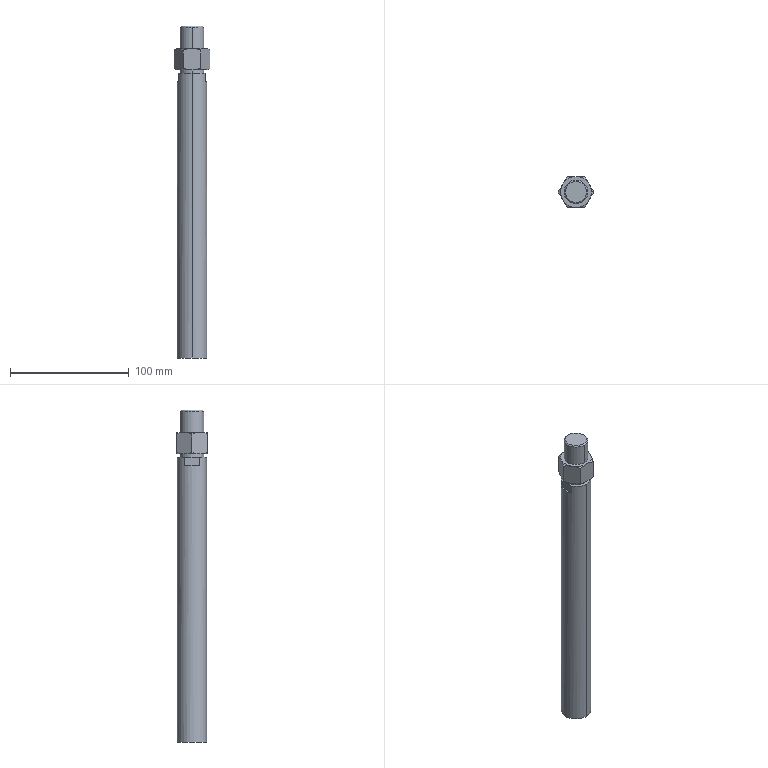Part | SolidWorks | features ICE 4, Chamfer 1, Revolution 1 | 1 solid | 36 faces | box 30 x 25.981 x 280 mm | volume 135007 mm3 | cone 15 | plane 15 | cylinder 6 | commonest cylinder face diameters 20 x4 25 x2
STEP:
#1=CARTESIAN_POINT('',(0.,-9.,318.));
#2=VERTEX_POINT('',#1);
#3=CARTESIAN_POINT('',(0.,9.,318.));
#4=VERTEX_POINT('',#3);
#5=CARTESIAN_POINT('',(0.,0.,318.));
#6=DIRECTION('',(0.,0.,1.));
#7=DIRECTION('',(0.,1.,0.));
#8=AXIS2_PLACEMENT_3D('',#5,#6,#7);
#9=CIRCLE('',#8,9.);
#10=EDGE_CURVE('',#2,#4,#9,.T.);
#11=ORIENTED_EDGE('',*,*,#10,.F.);
#12=CARTESIAN_POINT('',(0.,-10.,317.));
#13=VERTEX_POINT('',#12);
#14=CARTESIAN_POINT('',(0.,-9.,318.));
#15=DIRECTION('',(0.,-0.7071,-0.7071));
#16=VECTOR('',#15,1000.);
#17=LINE('',#14,#16);
#18=EDGE_CURVE('',#2,#13,#17,.T.);
#19=ORIENTED_EDGE('',*,*,#18,.T.);
#20=CARTESIAN_POINT('',(0.,10.,317.));
#21=VERTEX_POINT('',#20);
#22=CARTESIAN_POINT('',(0.,0.,317.));
#23=DIRECTION('',(0.,0.,-1.));
#24=DIRECTION('',(0.,1.,0.));
#25=AXIS2_PLACEMENT_3D('',#22,#23,#24);
#26=CIRCLE('',#25,10.);
#27=EDGE_CURVE('',#21,#13,#26,.T.);
#28=ORIENTED_EDGE('',*,*,#27,.F.);
#29=CARTESIAN_POINT('',(0.,9.,318.));
#30=DIRECTION('',(0.,0.7071,-0.7071));
#31=VECTOR('',#30,1000.);
#32=LINE('',#29,#31);
#33=EDGE_CURVE('',#4,#21,#32,.T.);
#34=ORIENTED_EDGE('',*,*,#33,.F.);
#35=EDGE_LOOP('',(#11,#19,#28,#34));
#36=FACE_OUTER_BOUND('',#35,.T.);
#37=CARTESIAN_POINT('',(0.,0.,318.));
#38=DIRECTION('',(0.,0.,-1.));
#39=DIRECTION('',(0.,1.,0.));
#40=AXIS2_PLACEMENT_3D('',#37,#38,#39);
#41=CONICAL_SURFACE('',#40,9.,0.7854);
#42=ADVANCED_FACE('',(#36),#41,.T.);
#43=CARTESIAN_POINT('',(0.,-10.,278.));
#44=VERTEX_POINT('',#43);
#45=CARTESIAN_POINT('',(0.,10.,278.));
#46=VERTEX_POINT('',#45);
#47=CARTESIAN_POINT('',(0.,0.,278.));
#48=DIRECTION('',(0.,0.,1.));
#49=DIRECTION('',(0.,-1.,0.));
#50=AXIS2_PLACEMENT_3D('',#47,#48,#49);
#51=CIRCLE('',#50,10.);
#52=EDGE_CURVE('',#44,#46,#51,.T.);
#53=ORIENTED_EDGE('',*,*,#52,.T.);
#54=CARTESIAN_POINT('',(0.,10.,281.));
#55=VERTEX_POINT('',#54);
#56=CARTESIAN_POINT('',(0.,10.,318.));
#57=DIRECTION('',(0.,0.,1.));
#58=VECTOR('',#57,1000.);
#59=LINE('',#56,#58);
#60=EDGE_CURVE('',#46,#55,#59,.T.);
#61=ORIENTED_EDGE('',*,*,#60,.T.);
#62=CARTESIAN_POINT('',(0.,-10.,281.));
#63=VERTEX_POINT('',#62);
#64=CARTESIAN_POINT('',(0.,0.,281.));
#65=DIRECTION('',(0.,0.,1.));
#66=DIRECTION('',(0.,-1.,0.));
#67=AXIS2_PLACEMENT_3D('',#64,#65,#66);
#68=CIRCLE('',#67,10.);
#69=EDGE_CURVE('',#63,#55,#68,.T.);
#70=ORIENTED_EDGE('',*,*,#69,.F.);
#71=CARTESIAN_POINT('',(0.,-10.,318.));
#72=DIRECTION('',(0.,0.,1.));
#73=VECTOR('',#72,1000.);
#74=LINE('',#71,#73);
#75=EDGE_CURVE('',#44,#63,#74,.T.);
#76=ORIENTED_EDGE('',*,*,#75,.F.);
#77=EDGE_LOOP('',(#53,#61,#70,#76));
#78=FACE_OUTER_BOUND('',#77,.T.);
#79=CARTESIAN_POINT('',(0.,0.,318.));
#80=DIRECTION('',(0.,0.,1.));
#81=DIRECTION('',(0.,-1.,0.));
#82=AXIS2_PLACEMENT_3D('',#79,#80,#81);
#83=CYLINDRICAL_SURFACE('',#82,10.);
#84=ADVANCED_FACE('',(#78),#83,.T.);
#85=CARTESIAN_POINT('',(0.,-12.5,38.));
#86=VERTEX_POINT('',#85);
#87=CARTESIAN_POINT('',(0.,12.5,38.));
#88=VERTEX_POINT('',#87);
#89=CARTESIAN_POINT('',(0.,0.,38.));
#90=DIRECTION('',(0.,0.,1.));
#91=DIRECTION('',(0.,-1.,0.));
#92=AXIS2_PLACEMENT_3D('',#89,#90,#91);
#93=CIRCLE('',#92,12.5);
#94=EDGE_CURVE('',#86,#88,#93,.T.);
#95=ORIENTED_EDGE('',*,*,#94,.T.);
#96=CARTESIAN_POINT('',(0.,12.5,278.));
#97=VERTEX_POINT('',#96);
#98=CARTESIAN_POINT('',(0.,12.5,318.));
#99=DIRECTION('',(0.,0.,1.));
#100=VECTOR('',#99,1000.);
#101=LINE('',#98,#100);
#102=EDGE_CURVE('',#88,#97,#101,.T.);
#103=ORIENTED_EDGE('',*,*,#102,.T.);
#104=CARTESIAN_POINT('',(11.,5.937,278.));
#105=VERTEX_POINT('',#104);
#106=CARTESIAN_POINT('',(0.,0.,278.));
#107=DIRECTION('',(0.,0.,1.));
#108=DIRECTION('',(0.,-1.,0.));
#109=AXIS2_PLACEMENT_3D('',#106,#107,#108);
#110=CIRCLE('',#109,12.5);
#111=EDGE_CURVE('',#105,#97,#110,.T.);
#112=ORIENTED_EDGE('',*,*,#111,.F.);
#113=CARTESIAN_POINT('',(11.,5.937,271.));
#114=VERTEX_POINT('',#113);
#115=CARTESIAN_POINT('',(11.,5.937,318.));
#116=DIRECTION('',(0.,0.,-1.));
#117=VECTOR('',#116,1000.);
#118=LINE('',#115,#117);
#119=EDGE_CURVE('',#105,#114,#118,.T.);
#120=ORIENTED_EDGE('',*,*,#119,.T.);
#121=CARTESIAN_POINT('',(11.,-5.937,271.));
#122=VERTEX_POINT('',#121);
#123=CARTESIAN_POINT('',(0.,0.,271.));
#124=DIRECTION('',(0.,0.,-1.));
#125=DIRECTION('',(-1.,0.,0.));
#126=AXIS2_PLACEMENT_3D('',#123,#124,#125);
#127=CIRCLE('',#126,12.5);
#128=EDGE_CURVE('',#114,#122,#127,.T.);
#129=ORIENTED_EDGE('',*,*,#128,.T.);
#130=CARTESIAN_POINT('',(11.,-5.937,278.));
#131=VERTEX_POINT('',#130);
#132=CARTESIAN_POINT('',(11.,-5.937,318.));
#133=DIRECTION('',(0.,0.,1.));
#134=VECTOR('',#133,1000.);
#135=LINE('',#132,#134);
#136=EDGE_CURVE('',#122,#131,#135,.T.);
#137=ORIENTED_EDGE('',*,*,#136,.T.);
#138=CARTESIAN_POINT('',(0.,-12.5,278.));
#139=VERTEX_POINT('',#138);
#140=CARTESIAN_POINT('',(0.,0.,278.));
#141=DIRECTION('',(0.,0.,1.));
#142=DIRECTION('',(0.,-1.,0.));
#143=AXIS2_PLACEMENT_3D('',#140,#141,#142);
#144=CIRCLE('',#143,12.5);
#145=EDGE_CURVE('',#139,#131,#144,.T.);
#146=ORIENTED_EDGE('',*,*,#145,.F.);
#147=CARTESIAN_POINT('',(0.,-12.5,318.));
#148=DIRECTION('',(0.,0.,1.));
#149=VECTOR('',#148,1000.);
#150=LINE('',#147,#149);
#151=EDGE_CURVE('',#86,#139,#150,.T.);
#152=ORIENTED_EDGE('',*,*,#151,.F.);
#153=EDGE_LOOP('',(#95,#103,#112,#120,#129,#137,#146,#152));
#154=FACE_OUTER_BOUND('',#153,.T.);
#155=CARTESIAN_POINT('',(0.,0.,318.));
#156=DIRECTION('',(0.,0.,1.));
#157=DIRECTION('',(0.,-1.,0.));
#158=AXIS2_PLACEMENT_3D('',#155,#156,#157);
#159=CYLINDRICAL_SURFACE('',#158,12.5);
#160=ADVANCED_FACE('',(#154),#159,.T.);
#161=CARTESIAN_POINT('',(0.,-10.,299.));
#162=VERTEX_POINT('',#161);
#163=CARTESIAN_POINT('',(0.,10.,299.));
#164=VERTEX_POINT('',#163);
#165=CARTESIAN_POINT('',(0.,0.,299.));
#166=DIRECTION('',(0.,0.,1.));
#167=DIRECTION('',(0.,-1.,0.));
#168=AXIS2_PLACEMENT_3D('',#165,#166,#167);
#169=CIRCLE('',#168,10.);
#170=EDGE_CURVE('',#162,#164,#169,.T.);
#171=ORIENTED_EDGE('',*,*,#170,.T.);
#172=CARTESIAN_POINT('',(0.,10.,318.));
#173=DIRECTION('',(0.,0.,1.));
#174=VECTOR('',#173,1000.);
#175=LINE('',#172,#174);
#176=EDGE_CURVE('',#164,#21,#175,.T.);
#177=ORIENTED_EDGE('',*,*,#176,.T.);
#178=ORIENTED_EDGE('',*,*,#27,.T.);
#179=CARTESIAN_POINT('',(0.,-10.,318.));
#180=DIRECTION('',(0.,0.,1.));
#181=VECTOR('',#180,1000.);
#182=LINE('',#179,#181);
#183=EDGE_CURVE('',#162,#13,#182,.T.);
#184=ORIENTED_EDGE('',*,*,#183,.F.);
#185=EDGE_LOOP('',(#171,#177,#178,#184));
#186=FACE_OUTER_BOUND('',#185,.T.);
#187=CARTESIAN_POINT('',(0.,0.,318.));
#188=DIRECTION('',(0.,0.,1.));
#189=DIRECTION('',(0.,-1.,0.));
#190=AXIS2_PLACEMENT_3D('',#187,#188,#189);
#191=CYLINDRICAL_SURFACE('',#190,10.);
#192=ADVANCED_FACE('',(#186),#191,.T.);
#193=CARTESIAN_POINT('',(12.99,0.,299.));
#194=VERTEX_POINT('',#193);
#195=CARTESIAN_POINT('',(11.25,6.495,299.));
#196=VERTEX_POINT('',#195);
#197=CARTESIAN_POINT('',(0.,0.,299.));
#198=DIRECTION('',(0.,0.,1.));
#199=DIRECTION('',(0.,-1.,0.));
#200=AXIS2_PLACEMENT_3D('',#197,#198,#199);
#201=CIRCLE('',#200,12.99);
#202=EDGE_CURVE('',#194,#196,#201,.T.);
#203=ORIENTED_EDGE('',*,*,#202,.F.);
#204=CARTESIAN_POINT('',(15.,0.,297.84));
#205=VERTEX_POINT('',#204);
#206=CARTESIAN_POINT('',(12.99,0.,299.));
#207=DIRECTION('',(0.866,0.,-0.5));
#208=VECTOR('',#207,1000.);
#209=LINE('',#206,#208);
#210=EDGE_CURVE('',#194,#205,#209,.T.);
#211=ORIENTED_EDGE('',*,*,#210,.T.);
#212=CARTESIAN_POINT('',(11.25,6.495,299.));
#213=CARTESIAN_POINT('',(11.568,5.944,299.));
#214=CARTESIAN_POINT('',(11.888,5.39,298.973));
#215=CARTESIAN_POINT('',(12.52,4.295,298.866));
#216=CARTESIAN_POINT('',(12.834,3.751,298.788));
#217=CARTESIAN_POINT('',(13.771,2.129,298.485));
#218=CARTESIAN_POINT('',(14.388,1.06,298.193));
#219=CARTESIAN_POINT('',(15.,0.,297.84));
#220=B_SPLINE_CURVE_WITH_KNOTS('',3,(#212,#213,#214,#215,#216,#217,#218,#219),.UNSPECIFIED.,.F.,.F.,(4,2,2,4),(0.007589,0.009479,0.01137,0.01515),.UNSPECIFIED.);
#221=EDGE_CURVE('',#196,#205,#220,.T.);
#222=ORIENTED_EDGE('',*,*,#221,.F.);
#223=EDGE_LOOP('',(#203,#211,#222));
#224=FACE_OUTER_BOUND('',#223,.T.);
#225=CARTESIAN_POINT('',(0.,0.,299.));
#226=DIRECTION('',(0.,0.,-1.));
#227=DIRECTION('',(1.,0.,0.));
#228=AXIS2_PLACEMENT_3D('',#225,#226,#227);
#229=CONICAL_SURFACE('',#228,12.99,1.047);
#230=ADVANCED_FACE('',(#224),#229,.T.);
#231=CARTESIAN_POINT('',(15.,0.,282.16));
#232=VERTEX_POINT('',#231);
#233=CARTESIAN_POINT('',(15.,0.,238.149));
#234=DIRECTION('',(0.,0.,1.));
#235=VECTOR('',#234,1000.);
#236=LINE('',#233,#235);
#237=EDGE_CURVE('',#232,#205,#236,.T.);
#238=ORIENTED_EDGE('',*,*,#237,.F.);
#239=CARTESIAN_POINT('',(11.25,6.495,281.));
#240=VERTEX_POINT('',#239);
#241=CARTESIAN_POINT('',(15.,0.,282.16));
#242=CARTESIAN_POINT('',(14.387,1.063,281.806));
#243=CARTESIAN_POINT('',(13.769,2.133,281.514));
#244=CARTESIAN_POINT('',(12.52,4.296,281.111));
#245=CARTESIAN_POINT('',(11.889,5.389,281.));
#246=CARTESIAN_POINT('',(11.25,6.495,281.));
#247=B_SPLINE_CURVE_WITH_KNOTS('',3,(#241,#242,#243,#244,#245,#246),.UNSPECIFIED.,.F.,.F.,(4,2,4),(0.000000238,0.003795,0.007589),.UNSPECIFIED.);
#248=EDGE_CURVE('',#232,#240,#247,.T.);
#249=ORIENTED_EDGE('',*,*,#248,.T.);
#250=CARTESIAN_POINT('',(7.5,12.99,282.16));
#251=VERTEX_POINT('',#250);
#252=CARTESIAN_POINT('',(11.25,6.495,281.));
#253=CARTESIAN_POINT('',(10.932,7.046,281.));
#254=CARTESIAN_POINT('',(10.612,7.6,281.027));
#255=CARTESIAN_POINT('',(9.98,8.695,281.134));
#256=CARTESIAN_POINT('',(9.666,9.239,281.212));
#257=CARTESIAN_POINT('',(8.729,10.862,281.515));
#258=CARTESIAN_POINT('',(8.112,11.931,281.807));
#259=CARTESIAN_POINT('',(7.5,12.99,282.16));
#260=B_SPLINE_CURVE_WITH_KNOTS('',3,(#252,#253,#254,#255,#256,#257,#258,#259),.UNSPECIFIED.,.F.,.F.,(4,2,2,4),(0.007589,0.009479,0.01137,0.01515),.UNSPECIFIED.);
#261=EDGE_CURVE('',#240,#251,#260,.T.);
#262=ORIENTED_EDGE('',*,*,#261,.T.);
#263=CARTESIAN_POINT('',(7.5,12.99,297.84));
#264=VERTEX_POINT('',#263);
#265=CARTESIAN_POINT('',(7.5,12.99,238.149));
#266=DIRECTION('',(0.,0.,1.));
#267=VECTOR('',#266,1000.);
#268=LINE('',#265,#267);
#269=EDGE_CURVE('',#251,#264,#268,.T.);
#270=ORIENTED_EDGE('',*,*,#269,.T.);
#271=CARTESIAN_POINT('',(7.5,12.99,297.84));
#272=CARTESIAN_POINT('',(8.113,11.928,298.194));
#273=CARTESIAN_POINT('',(8.731,10.858,298.486));
#274=CARTESIAN_POINT('',(9.98,8.695,298.889));
#275=CARTESIAN_POINT('',(10.611,7.602,299.));
#276=CARTESIAN_POINT('',(11.25,6.495,299.));
#277=B_SPLINE_CURVE_WITH_KNOTS('',3,(#271,#272,#273,#274,#275,#276),.UNSPECIFIED.,.F.,.F.,(4,2,4),(0.000000238,0.003795,0.007589),.UNSPECIFIED.);
#278=EDGE_CURVE('',#264,#196,#277,.T.);
#279=ORIENTED_EDGE('',*,*,#278,.T.);
#280=ORIENTED_EDGE('',*,*,#221,.T.);
#281=EDGE_LOOP('',(#238,#249,#262,#270,#279,#280));
#282=FACE_OUTER_BOUND('',#281,.T.);
#283=CARTESIAN_POINT('',(15.,0.,238.149));
#284=DIRECTION('',(0.866,0.5,0.));
#285=DIRECTION('',(-0.5,0.866,0.));
#286=AXIS2_PLACEMENT_3D('',#283,#284,#285);
#287=PLANE('',#286);
#288=ADVANCED_FACE('',(#282),#287,.T.);
#289=CARTESIAN_POINT('',(7.5,-12.99,282.16));
#290=VERTEX_POINT('',#289);
#291=CARTESIAN_POINT('',(7.5,-12.99,297.84));
#292=VERTEX_POINT('',#291);
#293=CARTESIAN_POINT('',(7.5,-12.99,238.149));
#294=DIRECTION('',(0.,0.,1.));
#295=VECTOR('',#294,1000.);
#296=LINE('',#293,#295);
#297=EDGE_CURVE('',#290,#292,#296,.T.);
#298=ORIENTED_EDGE('',*,*,#297,.F.);
#299=CARTESIAN_POINT('',(11.25,-6.495,281.));
#300=VERTEX_POINT('',#299);
#301=CARTESIAN_POINT('',(7.5,-12.99,282.16));
#302=CARTESIAN_POINT('',(8.113,-11.928,281.806));
#303=CARTESIAN_POINT('',(8.731,-10.858,281.514));
#304=CARTESIAN_POINT('',(9.98,-8.695,281.111));
#305=CARTESIAN_POINT('',(10.611,-7.602,281.));
#306=CARTESIAN_POINT('',(11.25,-6.495,281.));
#307=B_SPLINE_CURVE_WITH_KNOTS('',3,(#301,#302,#303,#304,#305,#306),.UNSPECIFIED.,.F.,.F.,(4,2,4),(0.000000238,0.003795,0.007589),.UNSPECIFIED.);
#308=EDGE_CURVE('',#290,#300,#307,.T.);
#309=ORIENTED_EDGE('',*,*,#308,.T.);
#310=CARTESIAN_POINT('',(11.25,-6.495,281.));
#311=CARTESIAN_POINT('',(11.568,-5.944,281.));
#312=CARTESIAN_POINT('',(11.888,-5.39,281.027));
#313=CARTESIAN_POINT('',(12.52,-4.295,281.134));
#314=CARTESIAN_POINT('',(12.834,-3.751,281.212));
#315=CARTESIAN_POINT('',(13.771,-2.129,281.515));
#316=CARTESIAN_POINT('',(14.388,-1.06,281.807));
#317=CARTESIAN_POINT('',(15.,0.,282.16));
#318=B_SPLINE_CURVE_WITH_KNOTS('',3,(#310,#311,#312,#313,#314,#315,#316,#317),.UNSPECIFIED.,.F.,.F.,(4,2,2,4),(0.007589,0.009479,0.01137,0.01515),.UNSPECIFIED.);
#319=EDGE_CURVE('',#300,#232,#318,.T.);
#320=ORIENTED_EDGE('',*,*,#319,.T.);
#321=ORIENTED_EDGE('',*,*,#237,.T.);
#322=CARTESIAN_POINT('',(11.25,-6.495,299.));
#323=VERTEX_POINT('',#322);
#324=CARTESIAN_POINT('',(15.,0.,297.84));
#325=CARTESIAN_POINT('',(14.387,-1.063,298.194));
#326=CARTESIAN_POINT('',(13.769,-2.133,298.486));
#327=CARTESIAN_POINT('',(12.52,-4.296,298.889));
#328=CARTESIAN_POINT('',(11.889,-5.389,299.));
#329=CARTESIAN_POINT('',(11.25,-6.495,299.));
#330=B_SPLINE_CURVE_WITH_KNOTS('',3,(#324,#325,#326,#327,#328,#329),.UNSPECIFIED.,.F.,.F.,(4,2,4),(0.000000238,0.003795,0.007589),.UNSPECIFIED.);
#331=EDGE_CURVE('',#205,#323,#330,.T.);
#332=ORIENTED_EDGE('',*,*,#331,.T.);
#333=CARTESIAN_POINT('',(11.25,-6.495,299.));
#334=CARTESIAN_POINT('',(10.932,-7.046,299.));
#335=CARTESIAN_POINT('',(10.612,-7.6,298.973));
#336=CARTESIAN_POINT('',(9.98,-8.695,298.866));
#337=CARTESIAN_POINT('',(9.666,-9.239,298.788));
#338=CARTESIAN_POINT('',(8.729,-10.862,298.485));
#339=CARTESIAN_POINT('',(8.112,-11.931,298.193));
#340=CARTESIAN_POINT('',(7.5,-12.99,297.84));
#341=B_SPLINE_CURVE_WITH_KNOTS('',3,(#333,#334,#335,#336,#337,#338,#339,#340),.UNSPECIFIED.,.F.,.F.,(4,2,2,4),(0.007589,0.009479,0.01137,0.01515),.UNSPECIFIED.);
#342=EDGE_CURVE('',#323,#292,#341,.T.);
#343=ORIENTED_EDGE('',*,*,#342,.T.);
#344=EDGE_LOOP('',(#298,#309,#320,#321,#332,#343));
#345=FACE_OUTER_BOUND('',#344,.T.);
#346=CARTESIAN_POINT('',(7.5,-12.99,238.149));
#347=DIRECTION('',(0.866,-0.5,0.));
#348=DIRECTION('',(0.5,0.866,0.));
#349=AXIS2_PLACEMENT_3D('',#346,#347,#348);
#350=PLANE('',#349);
#351=ADVANCED_FACE('',(#345),#350,.T.);
#352=CARTESIAN_POINT('',(-7.5,-12.99,282.16));
#353=VERTEX_POINT('',#352);
#354=CARTESIAN_POINT('',(-7.5,-12.99,297.84));
#355=VERTEX_POINT('',#354);
#356=CARTESIAN_POINT('',(-7.5,-12.99,238.149));
#357=DIRECTION('',(0.,0.,1.));
#358=VECTOR('',#357,1000.);
#359=LINE('',#356,#358);
#360=EDGE_CURVE('',#353,#355,#359,.T.);
#361=ORIENTED_EDGE('',*,*,#360,.F.);
#362=CARTESIAN_POINT('',(0.,-12.99,281.));
#363=VERTEX_POINT('',#362);
#364=CARTESIAN_POINT('',(-7.5,-12.99,282.16));
#365=CARTESIAN_POINT('',(-6.889,-12.99,281.984));
#366=CARTESIAN_POINT('',(-6.271,-12.99,281.822));
#367=CARTESIAN_POINT('',(-5.028,-12.99,281.535));
#368=CARTESIAN_POINT('',(-4.405,-12.99,281.412));
#369=CARTESIAN_POINT('',(-2.528,-12.99,281.109));
#370=CARTESIAN_POINT('',(-1.269,-12.99,281.));
#371=CARTESIAN_POINT('',(0.,-12.99,281.));
#372=B_SPLINE_CURVE_WITH_KNOTS('',3,(#364,#365,#366,#367,#368,#369,#370,#371),.UNSPECIFIED.,.F.,.F.,(4,2,2,4),(0.01398,0.01588,0.01777,0.02157),.UNSPECIFIED.);
#373=EDGE_CURVE('',#353,#363,#372,.T.);
#374=ORIENTED_EDGE('',*,*,#373,.T.);
#375=CARTESIAN_POINT('',(0.,-12.99,281.));
#376=CARTESIAN_POINT('',(0.6351,-12.99,281.));
#377=CARTESIAN_POINT('',(1.274,-12.99,281.027));
#378=CARTESIAN_POINT('',(2.55,-12.99,281.134));
#379=CARTESIAN_POINT('',(3.182,-12.99,281.214));
#380=CARTESIAN_POINT('',(5.058,-12.99,281.519));
#381=CARTESIAN_POINT('',(6.287,-12.99,281.81));
#382=CARTESIAN_POINT('',(7.5,-12.99,282.16));
#383=B_SPLINE_CURVE_WITH_KNOTS('',3,(#375,#376,#377,#378,#379,#380,#381,#382),.UNSPECIFIED.,.F.,.F.,(4,2,2,4),(0.02157,0.02347,0.02537,0.02917),.UNSPECIFIED.);
#384=EDGE_CURVE('',#363,#290,#383,.T.);
#385=ORIENTED_EDGE('',*,*,#384,.T.);
#386=ORIENTED_EDGE('',*,*,#297,.T.);
#387=CARTESIAN_POINT('',(0.,-12.99,299.));
#388=VERTEX_POINT('',#387);
#389=CARTESIAN_POINT('',(7.5,-12.99,297.84));
#390=CARTESIAN_POINT('',(6.287,-12.99,298.19));
#391=CARTESIAN_POINT('',(5.058,-12.99,298.481));
#392=CARTESIAN_POINT('',(3.182,-12.99,298.786));
#393=CARTESIAN_POINT('',(2.55,-12.99,298.866));
#394=CARTESIAN_POINT('',(1.274,-12.99,298.973));
#395=CARTESIAN_POINT('',(0.6351,-12.99,299.));
#396=CARTESIAN_POINT('',(0.,-12.99,299.));
#397=B_SPLINE_CURVE_WITH_KNOTS('',3,(#389,#390,#391,#392,#393,#394,#395,#396),.UNSPECIFIED.,.F.,.F.,(4,2,2,4),(0.03988,0.04368,0.04558,0.04748),.UNSPECIFIED.);
#398=EDGE_CURVE('',#292,#388,#397,.T.);
#399=ORIENTED_EDGE('',*,*,#398,.T.);
#400=CARTESIAN_POINT('',(0.,-12.99,299.));
#401=CARTESIAN_POINT('',(-1.269,-12.99,299.));
#402=CARTESIAN_POINT('',(-2.528,-12.99,298.891));
#403=CARTESIAN_POINT('',(-4.405,-12.99,298.588));
#404=CARTESIAN_POINT('',(-5.028,-12.99,298.465));
#405=CARTESIAN_POINT('',(-6.271,-12.99,298.178));
#406=CARTESIAN_POINT('',(-6.889,-12.99,298.016));
#407=CARTESIAN_POINT('',(-7.5,-12.99,297.84));
#408=B_SPLINE_CURVE_WITH_KNOTS('',3,(#400,#401,#402,#403,#404,#405,#406,#407),.UNSPECIFIED.,.F.,.F.,(4,2,2,4),(0.04748,0.05128,0.05317,0.05507),.UNSPECIFIED.);
#409=EDGE_CURVE('',#388,#355,#408,.T.);
#410=ORIENTED_EDGE('',*,*,#409,.T.);
#411=EDGE_LOOP('',(#361,#374,#385,#386,#399,#410));
#412=FACE_OUTER_BOUND('',#411,.T.);
#413=CARTESIAN_POINT('',(-7.5,-12.99,238.149));
#414=DIRECTION('',(0.,-1.,0.));
#415=DIRECTION('',(1.,0.,0.));
#416=AXIS2_PLACEMENT_3D('',#413,#414,#415);
#417=PLANE('',#416);
#418=ADVANCED_FACE('',(#412),#417,.T.);
#419=CARTESIAN_POINT('',(-15.,0.,282.16));
#420=VERTEX_POINT('',#419);
#421=CARTESIAN_POINT('',(-15.,0.,297.84));
#422=VERTEX_POINT('',#421);
#423=CARTESIAN_POINT('',(-15.,0.,238.149));
#424=DIRECTION('',(0.,0.,1.));
#425=VECTOR('',#424,1000.);
#426=LINE('',#423,#425);
#427=EDGE_CURVE('',#420,#422,#426,.T.);
#428=ORIENTED_EDGE('',*,*,#427,.F.);
#429=CARTESIAN_POINT('',(-11.25,-6.495,281.));
#430=VERTEX_POINT('',#429);
#431=CARTESIAN_POINT('',(-15.,0.,282.16));
#432=CARTESIAN_POINT('',(-14.387,-1.063,281.806));
#433=CARTESIAN_POINT('',(-13.769,-2.133,281.514));
#434=CARTESIAN_POINT('',(-12.52,-4.296,281.111));
#435=CARTESIAN_POINT('',(-11.889,-5.389,281.));
#436=CARTESIAN_POINT('',(-11.25,-6.495,281.));
#437=B_SPLINE_CURVE_WITH_KNOTS('',3,(#431,#432,#433,#434,#435,#436),.UNSPECIFIED.,.F.,.F.,(4,2,4),(0.000000238,0.003795,0.007589),.UNSPECIFIED.);
#438=EDGE_CURVE('',#420,#430,#437,.T.);
#439=ORIENTED_EDGE('',*,*,#438,.T.);
#440=CARTESIAN_POINT('',(-11.25,-6.495,281.));
#441=CARTESIAN_POINT('',(-10.932,-7.046,281.));
#442=CARTESIAN_POINT('',(-10.612,-7.6,281.027));
#443=CARTESIAN_POINT('',(-9.98,-8.695,281.134));
#444=CARTESIAN_POINT('',(-9.666,-9.239,281.212));
#445=CARTESIAN_POINT('',(-8.729,-10.862,281.515));
#446=CARTESIAN_POINT('',(-8.112,-11.931,281.807));
#447=CARTESIAN_POINT('',(-7.5,-12.99,282.16));
#448=B_SPLINE_CURVE_WITH_KNOTS('',3,(#440,#441,#442,#443,#444,#445,#446,#447),.UNSPECIFIED.,.F.,.F.,(4,2,2,4),(0.007589,0.009479,0.01137,0.01515),.UNSPECIFIED.);
#449=EDGE_CURVE('',#430,#353,#448,.T.);
#450=ORIENTED_EDGE('',*,*,#449,.T.);
#451=ORIENTED_EDGE('',*,*,#360,.T.);
#452=CARTESIAN_POINT('',(-11.25,-6.495,299.));
#453=VERTEX_POINT('',#452);
#454=CARTESIAN_POINT('',(-7.5,-12.99,297.84));
#455=CARTESIAN_POINT('',(-8.113,-11.928,298.194));
#456=CARTESIAN_POINT('',(-8.731,-10.858,298.486));
#457=CARTESIAN_POINT('',(-9.98,-8.695,298.889));
#458=CARTESIAN_POINT('',(-10.611,-7.602,299.));
#459=CARTESIAN_POINT('',(-11.25,-6.495,299.));
#460=B_SPLINE_CURVE_WITH_KNOTS('',3,(#454,#455,#456,#457,#458,#459),.UNSPECIFIED.,.F.,.F.,(4,2,4),(0.000000238,0.003795,0.007589),.UNSPECIFIED.);
#461=EDGE_CURVE('',#355,#453,#460,.T.);
#462=ORIENTED_EDGE('',*,*,#461,.T.);
#463=CARTESIAN_POINT('',(-11.25,-6.495,299.));
#464=CARTESIAN_POINT('',(-11.568,-5.944,299.));
#465=CARTESIAN_POINT('',(-11.888,-5.39,298.973));
#466=CARTESIAN_POINT('',(-12.52,-4.295,298.866));
#467=CARTESIAN_POINT('',(-12.834,-3.751,298.788));
#468=CARTESIAN_POINT('',(-13.771,-2.129,298.485));
#469=CARTESIAN_POINT('',(-14.388,-1.06,298.193));
#470=CARTESIAN_POINT('',(-15.,0.,297.84));
#471=B_SPLINE_CURVE_WITH_KNOTS('',3,(#463,#464,#465,#466,#467,#468,#469,#470),.UNSPECIFIED.,.F.,.F.,(4,2,2,4),(0.007589,0.009479,0.01137,0.01515),.UNSPECIFIED.);
#472=EDGE_CURVE('',#453,#422,#471,.T.);
#473=ORIENTED_EDGE('',*,*,#472,.T.);
#474=EDGE_LOOP('',(#428,#439,#450,#451,#462,#473));
#475=FACE_OUTER_BOUND('',#474,.T.);
#476=CARTESIAN_POINT('',(-15.,0.,238.149));
#477=DIRECTION('',(-0.866,-0.5,0.));
#478=DIRECTION('',(0.5,-0.866,0.));
#479=AXIS2_PLACEMENT_3D('',#476,#477,#478);
#480=PLANE('',#479);
#481=ADVANCED_FACE('',(#475),#480,.T.);
#482=CARTESIAN_POINT('',(-7.5,12.99,282.16));
#483=VERTEX_POINT('',#482);
#484=CARTESIAN_POINT('',(-7.5,12.99,297.84));
#485=VERTEX_POINT('',#484);
#486=CARTESIAN_POINT('',(-7.5,12.99,238.149));
#487=DIRECTION('',(0.,0.,1.));
#488=VECTOR('',#487,1000.);
#489=LINE('',#486,#488);
#490=EDGE_CURVE('',#483,#485,#489,.T.);
#491=ORIENTED_EDGE('',*,*,#490,.F.);
#492=CARTESIAN_POINT('',(-11.25,6.495,281.));
#493=VERTEX_POINT('',#492);
#494=CARTESIAN_POINT('',(-7.5,12.99,282.16));
#495=CARTESIAN_POINT('',(-8.113,11.928,281.806));
#496=CARTESIAN_POINT('',(-8.731,10.858,281.514));
#497=CARTESIAN_POINT('',(-9.98,8.695,281.111));
#498=CARTESIAN_POINT('',(-10.611,7.602,281.));
#499=CARTESIAN_POINT('',(-11.25,6.495,281.));
#500=B_SPLINE_CURVE_WITH_KNOTS('',3,(#494,#495,#496,#497,#498,#499),.UNSPECIFIED.,.F.,.F.,(4,2,4),(0.000000238,0.003795,0.007589),.UNSPECIFIED.);
#501=EDGE_CURVE('',#483,#493,#500,.T.);
#502=ORIENTED_EDGE('',*,*,#501,.T.);
#503=CARTESIAN_POINT('',(-11.25,6.495,281.));
#504=CARTESIAN_POINT('',(-11.568,5.944,281.));
#505=CARTESIAN_POINT('',(-11.888,5.39,281.027));
#506=CARTESIAN_POINT('',(-12.52,4.295,281.134));
#507=CARTESIAN_POINT('',(-12.834,3.751,281.212));
#508=CARTESIAN_POINT('',(-13.771,2.129,281.515));
#509=CARTESIAN_POINT('',(-14.388,1.06,281.807));
#510=CARTESIAN_POINT('',(-15.,0.,282.16));
#511=B_SPLINE_CURVE_WITH_KNOTS('',3,(#503,#504,#505,#506,#507,#508,#509,#510),.UNSPECIFIED.,.F.,.F.,(4,2,2,4),(0.007589,0.009479,0.01137,0.01515),.UNSPECIFIED.);
#512=EDGE_CURVE('',#493,#420,#511,.T.);
#513=ORIENTED_EDGE('',*,*,#512,.T.);
#514=ORIENTED_EDGE('',*,*,#427,.T.);
#515=CARTESIAN_POINT('',(-11.25,6.495,299.));
#516=VERTEX_POINT('',#515);
#517=CARTESIAN_POINT('',(-15.,0.,297.84));
#518=CARTESIAN_POINT('',(-14.387,1.063,298.194));
#519=CARTESIAN_POINT('',(-13.769,2.133,298.486));
#520=CARTESIAN_POINT('',(-12.52,4.296,298.889));
#521=CARTESIAN_POINT('',(-11.889,5.389,299.));
#522=CARTESIAN_POINT('',(-11.25,6.495,299.));
#523=B_SPLINE_CURVE_WITH_KNOTS('',3,(#517,#518,#519,#520,#521,#522),.UNSPECIFIED.,.F.,.F.,(4,2,4),(0.000000238,0.003795,0.007589),.UNSPECIFIED.);
#524=EDGE_CURVE('',#422,#516,#523,.T.);
#525=ORIENTED_EDGE('',*,*,#524,.T.);
#526=CARTESIAN_POINT('',(-11.25,6.495,299.));
#527=CARTESIAN_POINT('',(-10.932,7.046,299.));
#528=CARTESIAN_POINT('',(-10.612,7.6,298.973));
#529=CARTESIAN_POINT('',(-9.98,8.695,298.866));
#530=CARTESIAN_POINT('',(-9.666,9.239,298.788));
#531=CARTESIAN_POINT('',(-8.729,10.862,298.485));
#532=CARTESIAN_POINT('',(-8.112,11.931,298.193));
#533=CARTESIAN_POINT('',(-7.5,12.99,297.84));
#534=B_SPLINE_CURVE_WITH_KNOTS('',3,(#526,#527,#528,#529,#530,#531,#532,#533),.UNSPECIFIED.,.F.,.F.,(4,2,2,4),(0.007589,0.009479,0.01137,0.01515),.UNSPECIFIED.);
#535=EDGE_CURVE('',#516,#485,#534,.T.);
#536=ORIENTED_EDGE('',*,*,#535,.T.);
#537=EDGE_LOOP('',(#491,#502,#513,#514,#525,#536));
#538=FACE_OUTER_BOUND('',#537,.T.);
#539=CARTESIAN_POINT('',(-7.5,12.99,238.149));
#540=DIRECTION('',(-0.866,0.5,0.));
#541=DIRECTION('',(-0.5,-0.866,0.));
#542=AXIS2_PLACEMENT_3D('',#539,#540,#541);
#543=PLANE('',#542);
#544=ADVANCED_FACE('',(#538),#543,.T.);
#545=ORIENTED_EDGE('',*,*,#269,.F.);
#546=CARTESIAN_POINT('',(0.,12.99,281.));
#547=VERTEX_POINT('',#546);
#548=CARTESIAN_POINT('',(7.5,12.99,282.16));
#549=CARTESIAN_POINT('',(6.287,12.99,281.81));
#550=CARTESIAN_POINT('',(5.058,12.99,281.519));
#551=CARTESIAN_POINT('',(3.182,12.99,281.214));
#552=CARTESIAN_POINT('',(2.55,12.99,281.134));
#553=CARTESIAN_POINT('',(1.274,12.99,281.027));
#554=CARTESIAN_POINT('',(0.6351,12.99,281.));
#555=CARTESIAN_POINT('',(0.,12.99,281.));
#556=B_SPLINE_CURVE_WITH_KNOTS('',3,(#548,#549,#550,#551,#552,#553,#554,#555),.UNSPECIFIED.,.F.,.F.,(4,2,2,4),(0.03988,0.04368,0.04558,0.04748),.UNSPECIFIED.);
#557=EDGE_CURVE('',#251,#547,#556,.T.);
#558=ORIENTED_EDGE('',*,*,#557,.T.);
#559=CARTESIAN_POINT('',(0.,12.99,281.));
#560=CARTESIAN_POINT('',(-1.269,12.99,281.));
#561=CARTESIAN_POINT('',(-2.528,12.99,281.109));
#562=CARTESIAN_POINT('',(-4.405,12.99,281.412));
#563=CARTESIAN_POINT('',(-5.028,12.99,281.535));
#564=CARTESIAN_POINT('',(-6.271,12.99,281.822));
#565=CARTESIAN_POINT('',(-6.889,12.99,281.984));
#566=CARTESIAN_POINT('',(-7.5,12.99,282.16));
#567=B_SPLINE_CURVE_WITH_KNOTS('',3,(#559,#560,#561,#562,#563,#564,#565,#566),.UNSPECIFIED.,.F.,.F.,(4,2,2,4),(0.04748,0.05128,0.05317,0.05507),.UNSPECIFIED.);
#568=EDGE_CURVE('',#547,#483,#567,.T.);
#569=ORIENTED_EDGE('',*,*,#568,.T.);
#570=ORIENTED_EDGE('',*,*,#490,.T.);
#571=CARTESIAN_POINT('',(0.,12.99,299.));
#572=VERTEX_POINT('',#571);
#573=CARTESIAN_POINT('',(-7.5,12.99,297.84));
#574=CARTESIAN_POINT('',(-6.889,12.99,298.016));
#575=CARTESIAN_POINT('',(-6.271,12.99,298.178));
#576=CARTESIAN_POINT('',(-5.028,12.99,298.465));
#577=CARTESIAN_POINT('',(-4.405,12.99,298.588));
#578=CARTESIAN_POINT('',(-2.528,12.99,298.891));
#579=CARTESIAN_POINT('',(-1.269,12.99,299.));
#580=CARTESIAN_POINT('',(0.,12.99,299.));
#581=B_SPLINE_CURVE_WITH_KNOTS('',3,(#573,#574,#575,#576,#577,#578,#579,#580),.UNSPECIFIED.,.F.,.F.,(4,2,2,4),(0.01398,0.01588,0.01777,0.02157),.UNSPECIFIED.);
#582=EDGE_CURVE('',#485,#572,#581,.T.);
#583=ORIENTED_EDGE('',*,*,#582,.T.);
#584=CARTESIAN_POINT('',(0.,12.99,299.));
#585=CARTESIAN_POINT('',(0.6351,12.99,299.));
#586=CARTESIAN_POINT('',(1.274,12.99,298.973));
#587=CARTESIAN_POINT('',(2.55,12.99,298.866));
#588=CARTESIAN_POINT('',(3.182,12.99,298.786));
#589=CARTESIAN_POINT('',(5.058,12.99,298.481));
#590=CARTESIAN_POINT('',(6.287,12.99,298.19));
#591=CARTESIAN_POINT('',(7.5,12.99,297.84));
#592=B_SPLINE_CURVE_WITH_KNOTS('',3,(#584,#585,#586,#587,#588,#589,#590,#591),.UNSPECIFIED.,.F.,.F.,(4,2,2,4),(0.02157,0.02347,0.02537,0.02917),.UNSPECIFIED.);
#593=EDGE_CURVE('',#572,#264,#592,.T.);
#594=ORIENTED_EDGE('',*,*,#593,.T.);
#595=EDGE_LOOP('',(#545,#558,#569,#570,#583,#594));
#596=FACE_OUTER_BOUND('',#595,.T.);
#597=CARTESIAN_POINT('',(7.5,12.99,238.149));
#598=DIRECTION('',(0.,1.,0.));
#599=DIRECTION('',(-1.,0.,0.));
#600=AXIS2_PLACEMENT_3D('',#597,#598,#599);
#601=PLANE('',#600);
#602=ADVANCED_FACE('',(#596),#601,.T.);
#603=CARTESIAN_POINT('',(0.,0.,299.));
#604=DIRECTION('',(0.,0.,1.));
#605=DIRECTION('',(0.,-1.,0.));
#606=AXIS2_PLACEMENT_3D('',#603,#604,#605);
#607=CIRCLE('',#606,12.99);
#608=EDGE_CURVE('',#453,#388,#607,.T.);
#609=ORIENTED_EDGE('',*,*,#608,.F.);
#610=ORIENTED_EDGE('',*,*,#461,.F.);
#611=ORIENTED_EDGE('',*,*,#409,.F.);
#612=EDGE_LOOP('',(#609,#610,#611));
#613=FACE_OUTER_BOUND('',#612,.T.);
#614=CARTESIAN_POINT('',(0.,0.,299.));
#615=DIRECTION('',(0.,0.,-1.));
#616=DIRECTION('',(1.,0.,0.));
#617=AXIS2_PLACEMENT_3D('',#614,#615,#616);
#618=CONICAL_SURFACE('',#617,12.99,1.047);
#619=ADVANCED_FACE('',(#613),#618,.T.);
#620=CARTESIAN_POINT('',(0.,0.,299.));
#621=DIRECTION('',(0.,0.,1.));
#622=DIRECTION('',(0.,-1.,0.));
#623=AXIS2_PLACEMENT_3D('',#620,#621,#622);
#624=CIRCLE('',#623,12.99);
#625=EDGE_CURVE('',#516,#453,#624,.T.);
#626=ORIENTED_EDGE('',*,*,#625,.F.);
#627=ORIENTED_EDGE('',*,*,#524,.F.);
#628=ORIENTED_EDGE('',*,*,#472,.F.);
#629=EDGE_LOOP('',(#626,#627,#628));
#630=FACE_OUTER_BOUND('',#629,.T.);
#631=CARTESIAN_POINT('',(0.,0.,299.));
#632=DIRECTION('',(0.,0.,-1.));
#633=DIRECTION('',(1.,0.,0.));
#634=AXIS2_PLACEMENT_3D('',#631,#632,#633);
#635=CONICAL_SURFACE('',#634,12.99,1.047);
#636=ADVANCED_FACE('',(#630),#635,.T.);
#637=CARTESIAN_POINT('',(0.,0.,299.));
#638=DIRECTION('',(0.,0.,1.));
#639=DIRECTION('',(0.,-1.,0.));
#640=AXIS2_PLACEMENT_3D('',#637,#638,#639);
#641=CIRCLE('',#640,12.99);
#642=EDGE_CURVE('',#572,#516,#641,.T.);
#643=ORIENTED_EDGE('',*,*,#642,.F.);
#644=ORIENTED_EDGE('',*,*,#582,.F.);
#645=ORIENTED_EDGE('',*,*,#535,.F.);
#646=EDGE_LOOP('',(#643,#644,#645));
#647=FACE_OUTER_BOUND('',#646,.T.);
#648=CARTESIAN_POINT('',(0.,0.,299.));
#649=DIRECTION('',(0.,0.,-1.));
#650=DIRECTION('',(1.,0.,0.));
#651=AXIS2_PLACEMENT_3D('',#648,#649,#650);
#652=CONICAL_SURFACE('',#651,12.99,1.047);
#653=ADVANCED_FACE('',(#647),#652,.T.);
#654=ORIENTED_EDGE('',*,*,#593,.F.);
#655=CARTESIAN_POINT('',(0.,0.,299.));
#656=DIRECTION('',(0.,0.,1.));
#657=DIRECTION('',(1.,0.,0.));
#658=AXIS2_PLACEMENT_3D('',#655,#656,#657);
#659=CIRCLE('',#658,12.99);
#660=EDGE_CURVE('',#196,#572,#659,.T.);
#661=ORIENTED_EDGE('',*,*,#660,.F.);
#662=ORIENTED_EDGE('',*,*,#278,.F.);
#663=EDGE_LOOP('',(#654,#661,#662));
#664=FACE_OUTER_BOUND('',#663,.T.);
#665=CARTESIAN_POINT('',(0.,0.,299.));
#666=DIRECTION('',(0.,0.,-1.));
#667=DIRECTION('',(1.,0.,0.));
#668=AXIS2_PLACEMENT_3D('',#665,#666,#667);
#669=CONICAL_SURFACE('',#668,12.99,1.047);
#670=ADVANCED_FACE('',(#664),#669,.T.);
#671=ORIENTED_EDGE('',*,*,#210,.F.);
#672=CARTESIAN_POINT('',(0.,0.,299.));
#673=DIRECTION('',(0.,0.,1.));
#674=DIRECTION('',(0.,-1.,0.));
#675=AXIS2_PLACEMENT_3D('',#672,#673,#674);
#676=CIRCLE('',#675,12.99);
#677=EDGE_CURVE('',#323,#194,#676,.T.);
#678=ORIENTED_EDGE('',*,*,#677,.F.);
#679=ORIENTED_EDGE('',*,*,#331,.F.);
#680=EDGE_LOOP('',(#671,#678,#679));
#681=FACE_OUTER_BOUND('',#680,.T.);
#682=CARTESIAN_POINT('',(0.,0.,299.));
#683=DIRECTION('',(0.,0.,-1.));
#684=DIRECTION('',(1.,0.,0.));
#685=AXIS2_PLACEMENT_3D('',#682,#683,#684);
#686=CONICAL_SURFACE('',#685,12.99,1.047);
#687=ADVANCED_FACE('',(#681),#686,.T.);
#688=CARTESIAN_POINT('',(0.,0.,299.));
#689=DIRECTION('',(0.,0.,1.));
#690=DIRECTION('',(0.,-1.,0.));
#691=AXIS2_PLACEMENT_3D('',#688,#689,#690);
#692=CIRCLE('',#691,12.99);
#693=EDGE_CURVE('',#388,#323,#692,.T.);
#694=ORIENTED_EDGE('',*,*,#693,.F.);
#695=ORIENTED_EDGE('',*,*,#398,.F.);
#696=ORIENTED_EDGE('',*,*,#342,.F.);
#697=EDGE_LOOP('',(#694,#695,#696));
#698=FACE_OUTER_BOUND('',#697,.T.);
#699=CARTESIAN_POINT('',(0.,0.,299.));
#700=DIRECTION('',(0.,0.,-1.));
#701=DIRECTION('',(1.,0.,0.));
#702=AXIS2_PLACEMENT_3D('',#699,#700,#701);
#703=CONICAL_SURFACE('',#702,12.99,1.047);
#704=ADVANCED_FACE('',(#698),#703,.T.);
#705=CARTESIAN_POINT('',(0.,0.,318.));
#706=DIRECTION('',(0.,0.,1.));
#707=DIRECTION('',(0.,1.,0.));
#708=AXIS2_PLACEMENT_3D('',#705,#706,#707);
#709=CIRCLE('',#708,9.);
#710=EDGE_CURVE('',#4,#2,#709,.T.);
#711=ORIENTED_EDGE('',*,*,#710,.T.);
#712=ORIENTED_EDGE('',*,*,#10,.T.);
#713=EDGE_LOOP('',(#711,#712));
#714=FACE_OUTER_BOUND('',#713,.T.);
#715=CARTESIAN_POINT('',(0.,0.,318.));
#716=DIRECTION('',(0.,0.,-1.));
#717=DIRECTION('',(0.,1.,0.));
#718=AXIS2_PLACEMENT_3D('',#715,#716,#717);
#719=PLANE('',#718);
#720=ADVANCED_FACE('',(#714),#719,.F.);
#721=ORIENTED_EDGE('',*,*,#176,.F.);
#722=CARTESIAN_POINT('',(0.,0.,299.));
#723=DIRECTION('',(0.,0.,1.));
#724=DIRECTION('',(0.,-1.,0.));
#725=AXIS2_PLACEMENT_3D('',#722,#723,#724);
#726=CIRCLE('',#725,10.);
#727=EDGE_CURVE('',#164,#162,#726,.T.);
#728=ORIENTED_EDGE('',*,*,#727,.T.);
#729=ORIENTED_EDGE('',*,*,#183,.T.);
#730=CARTESIAN_POINT('',(0.,0.,317.));
#731=DIRECTION('',(0.,0.,-1.));
#732=DIRECTION('',(0.,1.,0.));
#733=AXIS2_PLACEMENT_3D('',#730,#731,#732);
#734=CIRCLE('',#733,10.);
#735=EDGE_CURVE('',#13,#21,#734,.T.);
#736=ORIENTED_EDGE('',*,*,#735,.T.);
#737=EDGE_LOOP('',(#721,#728,#729,#736));
#738=FACE_OUTER_BOUND('',#737,.T.);
#739=CARTESIAN_POINT('',(0.,0.,318.));
#740=DIRECTION('',(0.,0.,1.));
#741=DIRECTION('',(0.,-1.,0.));
#742=AXIS2_PLACEMENT_3D('',#739,#740,#741);
#743=CYLINDRICAL_SURFACE('',#742,10.);
#744=ADVANCED_FACE('',(#738),#743,.T.);
#745=ORIENTED_EDGE('',*,*,#170,.F.);
#746=ORIENTED_EDGE('',*,*,#727,.F.);
#747=EDGE_LOOP('',(#745,#746));
#748=FACE_BOUND('',#747,.T.);
#749=ORIENTED_EDGE('',*,*,#608,.T.);
#750=ORIENTED_EDGE('',*,*,#693,.T.);
#751=ORIENTED_EDGE('',*,*,#677,.T.);
#752=ORIENTED_EDGE('',*,*,#202,.T.);
#753=ORIENTED_EDGE('',*,*,#660,.T.);
#754=ORIENTED_EDGE('',*,*,#642,.T.);
#755=ORIENTED_EDGE('',*,*,#625,.T.);
#756=EDGE_LOOP('',(#749,#750,#751,#752,#753,#754,#755));
#757=FACE_OUTER_BOUND('',#756,.T.);
#758=CARTESIAN_POINT('',(0.,0.,299.));
#759=DIRECTION('',(0.,0.,1.));
#760=DIRECTION('',(0.,-1.,0.));
#761=AXIS2_PLACEMENT_3D('',#758,#759,#760);
#762=PLANE('',#761);
#763=ADVANCED_FACE('',(#748,#757),#762,.T.);
#764=ORIENTED_EDGE('',*,*,#568,.F.);
#765=CARTESIAN_POINT('',(0.,0.,281.));
#766=DIRECTION('',(0.,0.,-1.));
#767=DIRECTION('',(0.,1.,0.));
#768=AXIS2_PLACEMENT_3D('',#765,#766,#767);
#769=CIRCLE('',#768,12.99);
#770=EDGE_CURVE('',#493,#547,#769,.T.);
#771=ORIENTED_EDGE('',*,*,#770,.F.);
#772=ORIENTED_EDGE('',*,*,#501,.F.);
#773=EDGE_LOOP('',(#764,#771,#772));
#774=FACE_OUTER_BOUND('',#773,.T.);
#775=CARTESIAN_POINT('',(0.,0.,281.));
#776=DIRECTION('',(0.,0.,1.));
#777=DIRECTION('',(0.,1.,0.));
#778=AXIS2_PLACEMENT_3D('',#775,#776,#777);
#779=CONICAL_SURFACE('',#778,12.99,1.047);
#780=ADVANCED_FACE('',(#774),#779,.T.);
#781=ORIENTED_EDGE('',*,*,#512,.F.);
#782=CARTESIAN_POINT('',(0.,0.,281.));
#783=DIRECTION('',(0.,0.,-1.));
#784=DIRECTION('',(0.,1.,0.));
#785=AXIS2_PLACEMENT_3D('',#782,#783,#784);
#786=CIRCLE('',#785,12.99);
#787=EDGE_CURVE('',#430,#493,#786,.T.);
#788=ORIENTED_EDGE('',*,*,#787,.F.);
#789=ORIENTED_EDGE('',*,*,#438,.F.);
#790=EDGE_LOOP('',(#781,#788,#789));
#791=FACE_OUTER_BOUND('',#790,.T.);
#792=CARTESIAN_POINT('',(0.,0.,281.));
#793=DIRECTION('',(0.,0.,1.));
#794=DIRECTION('',(0.,1.,0.));
#795=AXIS2_PLACEMENT_3D('',#792,#793,#794);
#796=CONICAL_SURFACE('',#795,12.99,1.047);
#797=ADVANCED_FACE('',(#791),#796,.T.);
#798=ORIENTED_EDGE('',*,*,#449,.F.);
#799=CARTESIAN_POINT('',(0.,0.,281.));
#800=DIRECTION('',(0.,0.,-1.));
#801=DIRECTION('',(0.,1.,0.));
#802=AXIS2_PLACEMENT_3D('',#799,#800,#801);
#803=CIRCLE('',#802,12.99);
#804=EDGE_CURVE('',#363,#430,#803,.T.);
#805=ORIENTED_EDGE('',*,*,#804,.F.);
#806=ORIENTED_EDGE('',*,*,#373,.F.);
#807=EDGE_LOOP('',(#798,#805,#806));
#808=FACE_OUTER_BOUND('',#807,.T.);
#809=CARTESIAN_POINT('',(0.,0.,281.));
#810=DIRECTION('',(0.,0.,1.));
#811=DIRECTION('',(0.,1.,0.));
#812=AXIS2_PLACEMENT_3D('',#809,#810,#811);
#813=CONICAL_SURFACE('',#812,12.99,1.047);
#814=ADVANCED_FACE('',(#808),#813,.T.);
#815=CARTESIAN_POINT('',(0.,0.,281.));
#816=DIRECTION('',(0.,0.,-1.));
#817=DIRECTION('',(0.,1.,0.));
#818=AXIS2_PLACEMENT_3D('',#815,#816,#817);
#819=CIRCLE('',#818,12.99);
#820=EDGE_CURVE('',#300,#363,#819,.T.);
#821=ORIENTED_EDGE('',*,*,#820,.F.);
#822=ORIENTED_EDGE('',*,*,#308,.F.);
#823=ORIENTED_EDGE('',*,*,#384,.F.);
#824=EDGE_LOOP('',(#821,#822,#823));
#825=FACE_OUTER_BOUND('',#824,.T.);
#826=CARTESIAN_POINT('',(0.,0.,281.));
#827=DIRECTION('',(0.,0.,1.));
#828=DIRECTION('',(0.,1.,0.));
#829=AXIS2_PLACEMENT_3D('',#826,#827,#828);
#830=CONICAL_SURFACE('',#829,12.99,1.047);
#831=ADVANCED_FACE('',(#825),#830,.T.);
#832=CARTESIAN_POINT('',(0.,0.,281.));
#833=DIRECTION('',(0.,0.,-1.));
#834=DIRECTION('',(0.,1.,0.));
#835=AXIS2_PLACEMENT_3D('',#832,#833,#834);
#836=CIRCLE('',#835,12.99);
#837=EDGE_CURVE('',#240,#300,#836,.T.);
#838=ORIENTED_EDGE('',*,*,#837,.F.);
#839=ORIENTED_EDGE('',*,*,#248,.F.);
#840=ORIENTED_EDGE('',*,*,#319,.F.);
#841=EDGE_LOOP('',(#838,#839,#840));
#842=FACE_OUTER_BOUND('',#841,.T.);
#843=CARTESIAN_POINT('',(0.,0.,281.));
#844=DIRECTION('',(0.,0.,1.));
#845=DIRECTION('',(0.,1.,0.));
#846=AXIS2_PLACEMENT_3D('',#843,#844,#845);
#847=CONICAL_SURFACE('',#846,12.99,1.047);
#848=ADVANCED_FACE('',(#842),#847,.T.);
#849=CARTESIAN_POINT('',(0.,0.,281.));
#850=DIRECTION('',(0.,0.,-1.));
#851=DIRECTION('',(0.,1.,0.));
#852=AXIS2_PLACEMENT_3D('',#849,#850,#851);
#853=CIRCLE('',#852,12.99);
#854=EDGE_CURVE('',#547,#240,#853,.T.);
#855=ORIENTED_EDGE('',*,*,#854,.F.);
#856=ORIENTED_EDGE('',*,*,#557,.F.);
#857=ORIENTED_EDGE('',*,*,#261,.F.);
#858=EDGE_LOOP('',(#855,#856,#857));
#859=FACE_OUTER_BOUND('',#858,.T.);
#860=CARTESIAN_POINT('',(0.,0.,281.));
#861=DIRECTION('',(0.,0.,1.));
#862=DIRECTION('',(0.,1.,0.));
#863=AXIS2_PLACEMENT_3D('',#860,#861,#862);
#864=CONICAL_SURFACE('',#863,12.99,1.047);
#865=ADVANCED_FACE('',(#859),#864,.T.);
#866=ORIENTED_EDGE('',*,*,#94,.F.);
#867=CARTESIAN_POINT('',(0.,0.,38.));
#868=DIRECTION('',(0.,0.,1.));
#869=DIRECTION('',(0.,-1.,0.));
#870=AXIS2_PLACEMENT_3D('',#867,#868,#869);
#871=CIRCLE('',#870,12.5);
#872=EDGE_CURVE('',#88,#86,#871,.T.);
#873=ORIENTED_EDGE('',*,*,#872,.F.);
#874=EDGE_LOOP('',(#866,#873));
#875=FACE_OUTER_BOUND('',#874,.T.);
#876=CARTESIAN_POINT('',(0.,0.,38.));
#877=DIRECTION('',(0.,0.,-1.));
#878=DIRECTION('',(0.,1.,0.));
#879=AXIS2_PLACEMENT_3D('',#876,#877,#878);
#880=PLANE('',#879);
#881=ADVANCED_FACE('',(#875),#880,.T.);
#882=ORIENTED_EDGE('',*,*,#102,.F.);
#883=ORIENTED_EDGE('',*,*,#872,.T.);
#884=ORIENTED_EDGE('',*,*,#151,.T.);
#885=CARTESIAN_POINT('',(-11.,-5.937,278.));
#886=VERTEX_POINT('',#885);
#887=CARTESIAN_POINT('',(0.,0.,278.));
#888=DIRECTION('',(0.,0.,1.));
#889=DIRECTION('',(0.,-1.,0.));
#890=AXIS2_PLACEMENT_3D('',#887,#888,#889);
#891=CIRCLE('',#890,12.5);
#892=EDGE_CURVE('',#886,#139,#891,.T.);
#893=ORIENTED_EDGE('',*,*,#892,.F.);
#894=CARTESIAN_POINT('',(-11.,-5.937,271.));
#895=VERTEX_POINT('',#894);
#896=CARTESIAN_POINT('',(-11.,-5.937,318.));
#897=DIRECTION('',(0.,0.,-1.));
#898=VECTOR('',#897,1000.);
#899=LINE('',#896,#898);
#900=EDGE_CURVE('',#886,#895,#899,.T.);
#901=ORIENTED_EDGE('',*,*,#900,.T.);
#902=CARTESIAN_POINT('',(-11.,5.937,271.));
#903=VERTEX_POINT('',#902);
#904=CARTESIAN_POINT('',(0.,0.,271.));
#905=DIRECTION('',(0.,0.,1.));
#906=DIRECTION('',(1.,0.,0.));
#907=AXIS2_PLACEMENT_3D('',#904,#905,#906);
#908=CIRCLE('',#907,12.5);
#909=EDGE_CURVE('',#903,#895,#908,.T.);
#910=ORIENTED_EDGE('',*,*,#909,.F.);
#911=CARTESIAN_POINT('',(-11.,5.937,278.));
#912=VERTEX_POINT('',#911);
#913=CARTESIAN_POINT('',(-11.,5.937,318.));
#914=DIRECTION('',(0.,0.,1.));
#915=VECTOR('',#914,1000.);
#916=LINE('',#913,#915);
#917=EDGE_CURVE('',#903,#912,#916,.T.);
#918=ORIENTED_EDGE('',*,*,#917,.T.);
#919=CARTESIAN_POINT('',(0.,0.,278.));
#920=DIRECTION('',(0.,0.,1.));
#921=DIRECTION('',(0.,-1.,0.));
#922=AXIS2_PLACEMENT_3D('',#919,#920,#921);
#923=CIRCLE('',#922,12.5);
#924=EDGE_CURVE('',#97,#912,#923,.T.);
#925=ORIENTED_EDGE('',*,*,#924,.F.);
#926=EDGE_LOOP('',(#882,#883,#884,#893,#901,#910,#918,#925));
#927=FACE_OUTER_BOUND('',#926,.T.);
#928=CARTESIAN_POINT('',(0.,0.,318.));
#929=DIRECTION('',(0.,0.,1.));
#930=DIRECTION('',(0.,-1.,0.));
#931=AXIS2_PLACEMENT_3D('',#928,#929,#930);
#932=CYLINDRICAL_SURFACE('',#931,12.5);
#933=ADVANCED_FACE('',(#927),#932,.T.);
#934=ORIENTED_EDGE('',*,*,#52,.F.);
#935=CARTESIAN_POINT('',(0.,0.,278.));
#936=DIRECTION('',(0.,0.,1.));
#937=DIRECTION('',(0.,-1.,0.));
#938=AXIS2_PLACEMENT_3D('',#935,#936,#937);
#939=CIRCLE('',#938,10.);
#940=EDGE_CURVE('',#46,#44,#939,.T.);
#941=ORIENTED_EDGE('',*,*,#940,.F.);
#942=EDGE_LOOP('',(#934,#941));
#943=FACE_BOUND('',#942,.T.);
#944=ORIENTED_EDGE('',*,*,#892,.T.);
#945=ORIENTED_EDGE('',*,*,#145,.T.);
#946=CARTESIAN_POINT('',(11.,0.,278.));
#947=DIRECTION('',(0.,1.,0.));
#948=VECTOR('',#947,1000.);
#949=LINE('',#946,#948);
#950=EDGE_CURVE('',#131,#105,#949,.T.);
#951=ORIENTED_EDGE('',*,*,#950,.T.);
#952=ORIENTED_EDGE('',*,*,#111,.T.);
#953=ORIENTED_EDGE('',*,*,#924,.T.);
#954=CARTESIAN_POINT('',(-11.,0.,278.));
#955=DIRECTION('',(0.,-1.,0.));
#956=VECTOR('',#955,1000.);
#957=LINE('',#954,#956);
#958=EDGE_CURVE('',#912,#886,#957,.T.);
#959=ORIENTED_EDGE('',*,*,#958,.T.);
#960=EDGE_LOOP('',(#944,#945,#951,#952,#953,#959));
#961=FACE_OUTER_BOUND('',#960,.T.);
#962=CARTESIAN_POINT('',(0.,0.,278.));
#963=DIRECTION('',(0.,0.,-1.));
#964=DIRECTION('',(0.,1.,0.));
#965=AXIS2_PLACEMENT_3D('',#962,#963,#964);
#966=PLANE('',#965);
#967=ADVANCED_FACE('',(#943,#961),#966,.F.);
#968=ORIENTED_EDGE('',*,*,#60,.F.);
#969=ORIENTED_EDGE('',*,*,#940,.T.);
#970=ORIENTED_EDGE('',*,*,#75,.T.);
#971=CARTESIAN_POINT('',(0.,0.,281.));
#972=DIRECTION('',(0.,0.,1.));
#973=DIRECTION('',(0.,-1.,0.));
#974=AXIS2_PLACEMENT_3D('',#971,#972,#973);
#975=CIRCLE('',#974,10.);
#976=EDGE_CURVE('',#55,#63,#975,.T.);
#977=ORIENTED_EDGE('',*,*,#976,.F.);
#978=EDGE_LOOP('',(#968,#969,#970,#977));
#979=FACE_OUTER_BOUND('',#978,.T.);
#980=CARTESIAN_POINT('',(0.,0.,318.));
#981=DIRECTION('',(0.,0.,1.));
#982=DIRECTION('',(0.,-1.,0.));
#983=AXIS2_PLACEMENT_3D('',#980,#981,#982);
#984=CYLINDRICAL_SURFACE('',#983,10.);
#985=ADVANCED_FACE('',(#979),#984,.T.);
#986=ORIENTED_EDGE('',*,*,#69,.T.);
#987=ORIENTED_EDGE('',*,*,#976,.T.);
#988=EDGE_LOOP('',(#986,#987));
#989=FACE_BOUND('',#988,.T.);
#990=ORIENTED_EDGE('',*,*,#770,.T.);
#991=ORIENTED_EDGE('',*,*,#854,.T.);
#992=ORIENTED_EDGE('',*,*,#837,.T.);
#993=ORIENTED_EDGE('',*,*,#820,.T.);
#994=ORIENTED_EDGE('',*,*,#804,.T.);
#995=ORIENTED_EDGE('',*,*,#787,.T.);
#996=EDGE_LOOP('',(#990,#991,#992,#993,#994,#995));
#997=FACE_OUTER_BOUND('',#996,.T.);
#998=CARTESIAN_POINT('',(0.,0.,281.));
#999=DIRECTION('',(0.,0.,-1.));
#1000=DIRECTION('',(0.,1.,0.));
#1001=AXIS2_PLACEMENT_3D('',#998,#999,#1000);
#1002=PLANE('',#1001);
#1003=ADVANCED_FACE('',(#989,#997),#1002,.T.);
#1004=ORIENTED_EDGE('',*,*,#909,.T.);
#1005=CARTESIAN_POINT('',(-11.,12.99,271.));
#1006=DIRECTION('',(0.,1.,0.));
#1007=VECTOR('',#1006,1000.);
#1008=LINE('',#1005,#1007);
#1009=EDGE_CURVE('',#895,#903,#1008,.T.);
#1010=ORIENTED_EDGE('',*,*,#1009,.T.);
#1011=EDGE_LOOP('',(#1004,#1010));
#1012=FACE_OUTER_BOUND('',#1011,.T.);
#1013=CARTESIAN_POINT('',(-33.,12.99,271.));
#1014=DIRECTION('',(0.,0.,1.));
#1015=DIRECTION('',(1.,0.,0.));
#1016=AXIS2_PLACEMENT_3D('',#1013,#1014,#1015);
#1017=PLANE('',#1016);
#1018=ADVANCED_FACE('',(#1012),#1017,.T.);
#1019=ORIENTED_EDGE('',*,*,#1009,.F.);
#1020=ORIENTED_EDGE('',*,*,#900,.F.);
#1021=ORIENTED_EDGE('',*,*,#958,.F.);
#1022=ORIENTED_EDGE('',*,*,#917,.F.);
#1023=EDGE_LOOP('',(#1019,#1020,#1021,#1022));
#1024=FACE_OUTER_BOUND('',#1023,.T.);
#1025=CARTESIAN_POINT('',(-11.,12.99,271.));
#1026=DIRECTION('',(1.,0.,0.));
#1027=DIRECTION('',(0.,0.,-1.));
#1028=AXIS2_PLACEMENT_3D('',#1025,#1026,#1027);
#1029=PLANE('',#1028);
#1030=ADVANCED_FACE('',(#1024),#1029,.F.);
#1031=CARTESIAN_POINT('',(11.,12.99,271.));
#1032=DIRECTION('',(0.,-1.,0.));
#1033=VECTOR('',#1032,1000.);
#1034=LINE('',#1031,#1033);
#1035=EDGE_CURVE('',#114,#122,#1034,.T.);
#1036=ORIENTED_EDGE('',*,*,#1035,.T.);
#1037=ORIENTED_EDGE('',*,*,#128,.F.);
#1038=EDGE_LOOP('',(#1036,#1037));
#1039=FACE_OUTER_BOUND('',#1038,.T.);
#1040=CARTESIAN_POINT('',(33.,12.99,271.));
#1041=DIRECTION('',(0.,0.,-1.));
#1042=DIRECTION('',(-1.,0.,0.));
#1043=AXIS2_PLACEMENT_3D('',#1040,#1041,#1042);
#1044=PLANE('',#1043);
#1045=ADVANCED_FACE('',(#1039),#1044,.F.);
#1046=ORIENTED_EDGE('',*,*,#1035,.F.);
#1047=ORIENTED_EDGE('',*,*,#119,.F.);
#1048=ORIENTED_EDGE('',*,*,#950,.F.);
#1049=ORIENTED_EDGE('',*,*,#136,.F.);
#1050=EDGE_LOOP('',(#1046,#1047,#1048,#1049));
#1051=FACE_OUTER_BOUND('',#1050,.T.);
#1052=CARTESIAN_POINT('',(11.,12.99,271.));
#1053=DIRECTION('',(-1.,0.,0.));
#1054=DIRECTION('',(0.,0.,1.));
#1055=AXIS2_PLACEMENT_3D('',#1052,#1053,#1054);
#1056=PLANE('',#1055);
#1057=ADVANCED_FACE('',(#1051),#1056,.F.);
#1058=ORIENTED_EDGE('',*,*,#18,.F.);
#1059=ORIENTED_EDGE('',*,*,#710,.F.);
#1060=ORIENTED_EDGE('',*,*,#33,.T.);
#1061=ORIENTED_EDGE('',*,*,#735,.F.);
#1062=EDGE_LOOP('',(#1058,#1059,#1060,#1061));
#1063=FACE_OUTER_BOUND('',#1062,.T.);
#1064=CARTESIAN_POINT('',(0.,0.,318.));
#1065=DIRECTION('',(0.,0.,-1.));
#1066=DIRECTION('',(0.,1.,0.));
#1067=AXIS2_PLACEMENT_3D('',#1064,#1065,#1066);
#1068=CONICAL_SURFACE('',#1067,9.,0.7854);
#1069=ADVANCED_FACE('',(#1063),#1068,.T.);
#1070=CLOSED_SHELL('',(#42,#84,#160,#192,#230,#288,#351,#418,#481,#544,#602,#619,#636,#653,#670,#687,#704,#720,#744,#763,#780,#797,#814,#831,#848,#865,#881,#933,#967,#985,#1003,#1018,#1030,#1045,#1057,#1069));
#1071=MANIFOLD_SOLID_BREP('',#1070);
#1072=CARTESIAN_POINT('',(0.,0.,0.));
#1073=DIRECTION('',(0.,0.,1.));
#1074=DIRECTION('',(1.,0.,0.));
#1075=AXIS2_PLACEMENT_3D('',#1072,#1073,#1074);
#1076=(LENGTH_UNIT()NAMED_UNIT(*)SI_UNIT(.MILLI.,.METRE.));
#1077=UNCERTAINTY_MEASURE_WITH_UNIT(LENGTH_MEASURE(0.00001),#1076,'','');
#1078=(NAMED_UNIT(*)PLANE_ANGLE_UNIT()SI_UNIT($,.RADIAN.));
#1079=(NAMED_UNIT(*)SI_UNIT($,.STERADIAN.)SOLID_ANGLE_UNIT());
#1080=(GEOMETRIC_REPRESENTATION_CONTEXT(3)GLOBAL_UNCERTAINTY_ASSIGNED_CONTEXT((#1077))GLOBAL_UNIT_ASSIGNED_CONTEXT((#1076,#1078,#1079))REPRESENTATION_CONTEXT('',''));
#1081=ADVANCED_BREP_SHAPE_REPRESENTATION('',(#1071,#1075),#1080);